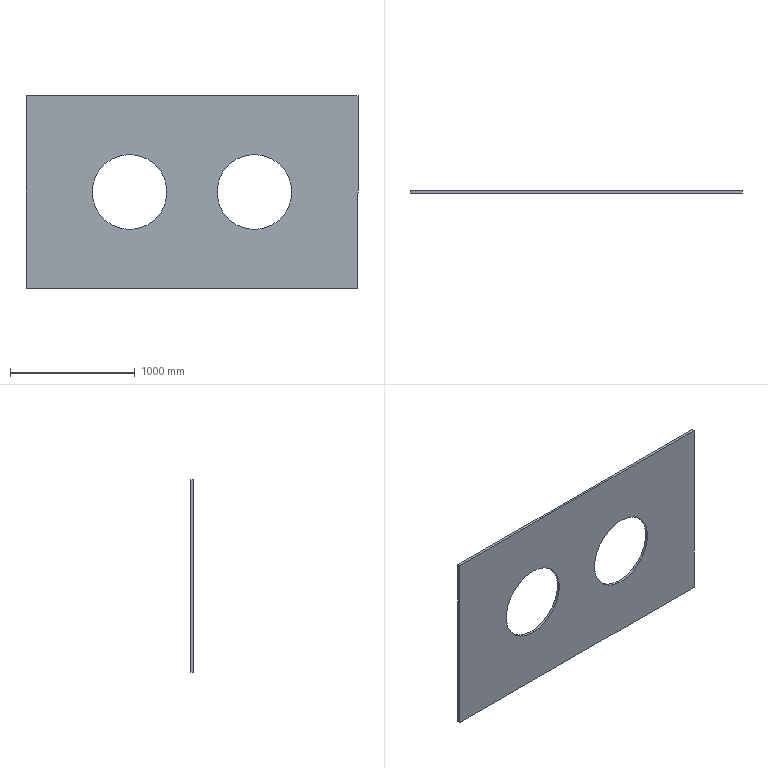Part | STEP file | 果蔬烘干机框架-105 | 1 solid | 10 faces | box 2660 x 20 x 1540 mm | volume 70618266 mm3 | plane 6 | cylinder 4 | commonest cylinder face diameters 600 x4
STEP:
#1=CARTESIAN_POINT('',(-500.,0.,-300.));
#2=VERTEX_POINT('',#1);
#3=CARTESIAN_POINT('',(-500.,0.,300.));
#4=VERTEX_POINT('',#3);
#5=CARTESIAN_POINT('',(-500.,0.,0.));
#6=DIRECTION('',(0.,1.,0.));
#7=DIRECTION('',(0.,0.,1.));
#8=AXIS2_PLACEMENT_3D('',#5,#6,#7);
#9=CIRCLE('',#8,300.);
#10=EDGE_CURVE('',#2,#4,#9,.T.);
#11=ORIENTED_EDGE('',*,*,#10,.F.);
#12=CARTESIAN_POINT('',(-500.,20.,-300.));
#13=VERTEX_POINT('',#12);
#14=CARTESIAN_POINT('',(-500.,0.,-300.));
#15=DIRECTION('',(0.,1.,0.));
#16=VECTOR('',#15,1000.);
#17=LINE('',#14,#16);
#18=EDGE_CURVE('',#2,#13,#17,.T.);
#19=ORIENTED_EDGE('',*,*,#18,.T.);
#20=CARTESIAN_POINT('',(-500.,20.,300.));
#21=VERTEX_POINT('',#20);
#22=CARTESIAN_POINT('',(-500.,20.,0.));
#23=DIRECTION('',(0.,1.,0.));
#24=DIRECTION('',(0.,0.,1.));
#25=AXIS2_PLACEMENT_3D('',#22,#23,#24);
#26=CIRCLE('',#25,300.);
#27=EDGE_CURVE('',#13,#21,#26,.T.);
#28=ORIENTED_EDGE('',*,*,#27,.T.);
#29=CARTESIAN_POINT('',(-500.,0.,300.));
#30=DIRECTION('',(0.,1.,0.));
#31=VECTOR('',#30,1000.);
#32=LINE('',#29,#31);
#33=EDGE_CURVE('',#4,#21,#32,.T.);
#34=ORIENTED_EDGE('',*,*,#33,.F.);
#35=EDGE_LOOP('',(#11,#19,#28,#34));
#36=FACE_OUTER_BOUND('',#35,.T.);
#37=CARTESIAN_POINT('',(-500.,0.,0.));
#38=DIRECTION('',(0.,1.,0.));
#39=DIRECTION('',(0.,0.,1.));
#40=AXIS2_PLACEMENT_3D('',#37,#38,#39);
#41=CYLINDRICAL_SURFACE('',#40,300.);
#42=ADVANCED_FACE('',(#36),#41,.F.);
#43=CARTESIAN_POINT('',(500.,0.,-300.));
#44=VERTEX_POINT('',#43);
#45=CARTESIAN_POINT('',(500.,0.,300.));
#46=VERTEX_POINT('',#45);
#47=CARTESIAN_POINT('',(500.,0.,0.));
#48=DIRECTION('',(0.,1.,0.));
#49=DIRECTION('',(0.,0.,1.));
#50=AXIS2_PLACEMENT_3D('',#47,#48,#49);
#51=CIRCLE('',#50,300.);
#52=EDGE_CURVE('',#44,#46,#51,.T.);
#53=ORIENTED_EDGE('',*,*,#52,.F.);
#54=CARTESIAN_POINT('',(500.,20.,-300.));
#55=VERTEX_POINT('',#54);
#56=CARTESIAN_POINT('',(500.,0.,-300.));
#57=DIRECTION('',(0.,1.,0.));
#58=VECTOR('',#57,1000.);
#59=LINE('',#56,#58);
#60=EDGE_CURVE('',#44,#55,#59,.T.);
#61=ORIENTED_EDGE('',*,*,#60,.T.);
#62=CARTESIAN_POINT('',(500.,20.,300.));
#63=VERTEX_POINT('',#62);
#64=CARTESIAN_POINT('',(500.,20.,0.));
#65=DIRECTION('',(0.,1.,0.));
#66=DIRECTION('',(0.,0.,1.));
#67=AXIS2_PLACEMENT_3D('',#64,#65,#66);
#68=CIRCLE('',#67,300.);
#69=EDGE_CURVE('',#55,#63,#68,.T.);
#70=ORIENTED_EDGE('',*,*,#69,.T.);
#71=CARTESIAN_POINT('',(500.,0.,300.));
#72=DIRECTION('',(0.,1.,0.));
#73=VECTOR('',#72,1000.);
#74=LINE('',#71,#73);
#75=EDGE_CURVE('',#46,#63,#74,.T.);
#76=ORIENTED_EDGE('',*,*,#75,.F.);
#77=EDGE_LOOP('',(#53,#61,#70,#76));
#78=FACE_OUTER_BOUND('',#77,.T.);
#79=CARTESIAN_POINT('',(500.,0.,0.));
#80=DIRECTION('',(0.,1.,0.));
#81=DIRECTION('',(0.,0.,1.));
#82=AXIS2_PLACEMENT_3D('',#79,#80,#81);
#83=CYLINDRICAL_SURFACE('',#82,300.);
#84=ADVANCED_FACE('',(#78),#83,.F.);
#85=CARTESIAN_POINT('',(1330.,0.,770.));
#86=VERTEX_POINT('',#85);
#87=CARTESIAN_POINT('',(1330.,0.,-770.));
#88=VERTEX_POINT('',#87);
#89=CARTESIAN_POINT('',(1330.,0.,-770.));
#90=DIRECTION('',(0.,0.,-1.));
#91=VECTOR('',#90,1000.);
#92=LINE('',#89,#91);
#93=EDGE_CURVE('',#86,#88,#92,.T.);
#94=ORIENTED_EDGE('',*,*,#93,.T.);
#95=CARTESIAN_POINT('',(1330.,20.,-770.));
#96=VERTEX_POINT('',#95);
#97=CARTESIAN_POINT('',(1330.,20.,-770.));
#98=DIRECTION('',(0.,-1.,0.));
#99=VECTOR('',#98,1000.);
#100=LINE('',#97,#99);
#101=EDGE_CURVE('',#96,#88,#100,.T.);
#102=ORIENTED_EDGE('',*,*,#101,.F.);
#103=CARTESIAN_POINT('',(1330.,20.,770.));
#104=VERTEX_POINT('',#103);
#105=CARTESIAN_POINT('',(1330.,20.,-770.));
#106=DIRECTION('',(0.,0.,-1.));
#107=VECTOR('',#106,1000.);
#108=LINE('',#105,#107);
#109=EDGE_CURVE('',#104,#96,#108,.T.);
#110=ORIENTED_EDGE('',*,*,#109,.F.);
#111=CARTESIAN_POINT('',(1330.,20.,770.));
#112=DIRECTION('',(0.,-1.,0.));
#113=VECTOR('',#112,1000.);
#114=LINE('',#111,#113);
#115=EDGE_CURVE('',#104,#86,#114,.T.);
#116=ORIENTED_EDGE('',*,*,#115,.T.);
#117=EDGE_LOOP('',(#94,#102,#110,#116));
#118=FACE_OUTER_BOUND('',#117,.T.);
#119=CARTESIAN_POINT('',(1330.,20.,-770.));
#120=DIRECTION('',(-1.,0.,0.));
#121=DIRECTION('',(0.,0.,1.));
#122=AXIS2_PLACEMENT_3D('',#119,#120,#121);
#123=PLANE('',#122);
#124=ADVANCED_FACE('',(#118),#123,.F.);
#125=CARTESIAN_POINT('',(-1330.,0.,-770.));
#126=VERTEX_POINT('',#125);
#127=CARTESIAN_POINT('',(-1330.,0.,-770.));
#128=DIRECTION('',(-1.,0.,0.));
#129=VECTOR('',#128,1000.);
#130=LINE('',#127,#129);
#131=EDGE_CURVE('',#88,#126,#130,.T.);
#132=ORIENTED_EDGE('',*,*,#131,.T.);
#133=CARTESIAN_POINT('',(-1330.,20.,-770.));
#134=VERTEX_POINT('',#133);
#135=CARTESIAN_POINT('',(-1330.,20.,-770.));
#136=DIRECTION('',(0.,-1.,0.));
#137=VECTOR('',#136,1000.);
#138=LINE('',#135,#137);
#139=EDGE_CURVE('',#134,#126,#138,.T.);
#140=ORIENTED_EDGE('',*,*,#139,.F.);
#141=CARTESIAN_POINT('',(-1330.,20.,-770.));
#142=DIRECTION('',(-1.,0.,0.));
#143=VECTOR('',#142,1000.);
#144=LINE('',#141,#143);
#145=EDGE_CURVE('',#96,#134,#144,.T.);
#146=ORIENTED_EDGE('',*,*,#145,.F.);
#147=ORIENTED_EDGE('',*,*,#101,.T.);
#148=EDGE_LOOP('',(#132,#140,#146,#147));
#149=FACE_OUTER_BOUND('',#148,.T.);
#150=CARTESIAN_POINT('',(-1330.,20.,-770.));
#151=DIRECTION('',(0.,0.,1.));
#152=DIRECTION('',(1.,0.,0.));
#153=AXIS2_PLACEMENT_3D('',#150,#151,#152);
#154=PLANE('',#153);
#155=ADVANCED_FACE('',(#149),#154,.F.);
#156=CARTESIAN_POINT('',(-1330.,0.,770.));
#157=VERTEX_POINT('',#156);
#158=CARTESIAN_POINT('',(-1330.,0.,-770.));
#159=DIRECTION('',(0.,0.,1.));
#160=VECTOR('',#159,1000.);
#161=LINE('',#158,#160);
#162=EDGE_CURVE('',#126,#157,#161,.T.);
#163=ORIENTED_EDGE('',*,*,#162,.T.);
#164=CARTESIAN_POINT('',(-1330.,20.,770.));
#165=VERTEX_POINT('',#164);
#166=CARTESIAN_POINT('',(-1330.,20.,770.));
#167=DIRECTION('',(0.,-1.,0.));
#168=VECTOR('',#167,1000.);
#169=LINE('',#166,#168);
#170=EDGE_CURVE('',#165,#157,#169,.T.);
#171=ORIENTED_EDGE('',*,*,#170,.F.);
#172=CARTESIAN_POINT('',(-1330.,20.,-770.));
#173=DIRECTION('',(0.,0.,1.));
#174=VECTOR('',#173,1000.);
#175=LINE('',#172,#174);
#176=EDGE_CURVE('',#134,#165,#175,.T.);
#177=ORIENTED_EDGE('',*,*,#176,.F.);
#178=ORIENTED_EDGE('',*,*,#139,.T.);
#179=EDGE_LOOP('',(#163,#171,#177,#178));
#180=FACE_OUTER_BOUND('',#179,.T.);
#181=CARTESIAN_POINT('',(-1330.,20.,-770.));
#182=DIRECTION('',(1.,0.,0.));
#183=DIRECTION('',(0.,0.,-1.));
#184=AXIS2_PLACEMENT_3D('',#181,#182,#183);
#185=PLANE('',#184);
#186=ADVANCED_FACE('',(#180),#185,.F.);
#187=CARTESIAN_POINT('',(-1330.,0.,770.));
#188=DIRECTION('',(1.,0.,0.));
#189=VECTOR('',#188,1000.);
#190=LINE('',#187,#189);
#191=EDGE_CURVE('',#157,#86,#190,.T.);
#192=ORIENTED_EDGE('',*,*,#191,.T.);
#193=ORIENTED_EDGE('',*,*,#115,.F.);
#194=CARTESIAN_POINT('',(-1330.,20.,770.));
#195=DIRECTION('',(1.,0.,0.));
#196=VECTOR('',#195,1000.);
#197=LINE('',#194,#196);
#198=EDGE_CURVE('',#165,#104,#197,.T.);
#199=ORIENTED_EDGE('',*,*,#198,.F.);
#200=ORIENTED_EDGE('',*,*,#170,.T.);
#201=EDGE_LOOP('',(#192,#193,#199,#200));
#202=FACE_OUTER_BOUND('',#201,.T.);
#203=CARTESIAN_POINT('',(-1330.,20.,770.));
#204=DIRECTION('',(0.,0.,-1.));
#205=DIRECTION('',(-1.,0.,0.));
#206=AXIS2_PLACEMENT_3D('',#203,#204,#205);
#207=PLANE('',#206);
#208=ADVANCED_FACE('',(#202),#207,.F.);
#209=CARTESIAN_POINT('',(-500.,20.,0.));
#210=DIRECTION('',(0.,1.,0.));
#211=DIRECTION('',(0.,0.,1.));
#212=AXIS2_PLACEMENT_3D('',#209,#210,#211);
#213=CIRCLE('',#212,300.);
#214=EDGE_CURVE('',#21,#13,#213,.T.);
#215=ORIENTED_EDGE('',*,*,#214,.F.);
#216=ORIENTED_EDGE('',*,*,#27,.F.);
#217=EDGE_LOOP('',(#215,#216));
#218=FACE_BOUND('',#217,.T.);
#219=CARTESIAN_POINT('',(500.,20.,0.));
#220=DIRECTION('',(0.,1.,0.));
#221=DIRECTION('',(0.,0.,1.));
#222=AXIS2_PLACEMENT_3D('',#219,#220,#221);
#223=CIRCLE('',#222,300.);
#224=EDGE_CURVE('',#63,#55,#223,.T.);
#225=ORIENTED_EDGE('',*,*,#224,.F.);
#226=ORIENTED_EDGE('',*,*,#69,.F.);
#227=EDGE_LOOP('',(#225,#226));
#228=FACE_BOUND('',#227,.T.);
#229=ORIENTED_EDGE('',*,*,#109,.T.);
#230=ORIENTED_EDGE('',*,*,#145,.T.);
#231=ORIENTED_EDGE('',*,*,#176,.T.);
#232=ORIENTED_EDGE('',*,*,#198,.T.);
#233=EDGE_LOOP('',(#229,#230,#231,#232));
#234=FACE_OUTER_BOUND('',#233,.T.);
#235=CARTESIAN_POINT('',(0.,20.,0.));
#236=DIRECTION('',(0.,1.,0.));
#237=DIRECTION('',(0.,0.,1.));
#238=AXIS2_PLACEMENT_3D('',#235,#236,#237);
#239=PLANE('',#238);
#240=ADVANCED_FACE('',(#218,#228,#234),#239,.T.);
#241=CARTESIAN_POINT('',(-500.,0.,0.));
#242=DIRECTION('',(0.,1.,0.));
#243=DIRECTION('',(0.,0.,1.));
#244=AXIS2_PLACEMENT_3D('',#241,#242,#243);
#245=CIRCLE('',#244,300.);
#246=EDGE_CURVE('',#4,#2,#245,.T.);
#247=ORIENTED_EDGE('',*,*,#246,.T.);
#248=ORIENTED_EDGE('',*,*,#10,.T.);
#249=EDGE_LOOP('',(#247,#248));
#250=FACE_BOUND('',#249,.T.);
#251=CARTESIAN_POINT('',(500.,0.,0.));
#252=DIRECTION('',(0.,1.,0.));
#253=DIRECTION('',(0.,0.,1.));
#254=AXIS2_PLACEMENT_3D('',#251,#252,#253);
#255=CIRCLE('',#254,300.);
#256=EDGE_CURVE('',#46,#44,#255,.T.);
#257=ORIENTED_EDGE('',*,*,#256,.T.);
#258=ORIENTED_EDGE('',*,*,#52,.T.);
#259=EDGE_LOOP('',(#257,#258));
#260=FACE_BOUND('',#259,.T.);
#261=ORIENTED_EDGE('',*,*,#93,.F.);
#262=ORIENTED_EDGE('',*,*,#191,.F.);
#263=ORIENTED_EDGE('',*,*,#162,.F.);
#264=ORIENTED_EDGE('',*,*,#131,.F.);
#265=EDGE_LOOP('',(#261,#262,#263,#264));
#266=FACE_OUTER_BOUND('',#265,.T.);
#267=CARTESIAN_POINT('',(0.,0.,0.));
#268=DIRECTION('',(0.,1.,0.));
#269=DIRECTION('',(0.,0.,1.));
#270=AXIS2_PLACEMENT_3D('',#267,#268,#269);
#271=PLANE('',#270);
#272=ADVANCED_FACE('',(#250,#260,#266),#271,.F.);
#273=ORIENTED_EDGE('',*,*,#60,.F.);
#274=ORIENTED_EDGE('',*,*,#256,.F.);
#275=ORIENTED_EDGE('',*,*,#75,.T.);
#276=ORIENTED_EDGE('',*,*,#224,.T.);
#277=EDGE_LOOP('',(#273,#274,#275,#276));
#278=FACE_OUTER_BOUND('',#277,.T.);
#279=CARTESIAN_POINT('',(500.,0.,0.));
#280=DIRECTION('',(0.,1.,0.));
#281=DIRECTION('',(0.,0.,1.));
#282=AXIS2_PLACEMENT_3D('',#279,#280,#281);
#283=CYLINDRICAL_SURFACE('',#282,300.);
#284=ADVANCED_FACE('',(#278),#283,.F.);
#285=ORIENTED_EDGE('',*,*,#18,.F.);
#286=ORIENTED_EDGE('',*,*,#246,.F.);
#287=ORIENTED_EDGE('',*,*,#33,.T.);
#288=ORIENTED_EDGE('',*,*,#214,.T.);
#289=EDGE_LOOP('',(#285,#286,#287,#288));
#290=FACE_OUTER_BOUND('',#289,.T.);
#291=CARTESIAN_POINT('',(-500.,0.,0.));
#292=DIRECTION('',(0.,1.,0.));
#293=DIRECTION('',(0.,0.,1.));
#294=AXIS2_PLACEMENT_3D('',#291,#292,#293);
#295=CYLINDRICAL_SURFACE('',#294,300.);
#296=ADVANCED_FACE('',(#290),#295,.F.);
#297=CLOSED_SHELL('',(#42,#84,#124,#155,#186,#208,#240,#272,#284,#296));
#298=MANIFOLD_SOLID_BREP('',#297);
#299=CARTESIAN_POINT('',(0.,0.,0.));
#300=DIRECTION('',(0.,0.,1.));
#301=DIRECTION('',(1.,0.,0.));
#302=AXIS2_PLACEMENT_3D('',#299,#300,#301);
#303=(LENGTH_UNIT()NAMED_UNIT(*)SI_UNIT(.MILLI.,.METRE.));
#304=UNCERTAINTY_MEASURE_WITH_UNIT(LENGTH_MEASURE(0.00001),#303,'','');
#305=(NAMED_UNIT(*)PLANE_ANGLE_UNIT()SI_UNIT($,.RADIAN.));
#306=(NAMED_UNIT(*)SI_UNIT($,.STERADIAN.)SOLID_ANGLE_UNIT());
#307=(GEOMETRIC_REPRESENTATION_CONTEXT(3)GLOBAL_UNCERTAINTY_ASSIGNED_CONTEXT((#304))GLOBAL_UNIT_ASSIGNED_CONTEXT((#303,#305,#306))REPRESENTATION_CONTEXT('',''));
#308=ADVANCED_BREP_SHAPE_REPRESENTATION('',(#298,#302),#307);